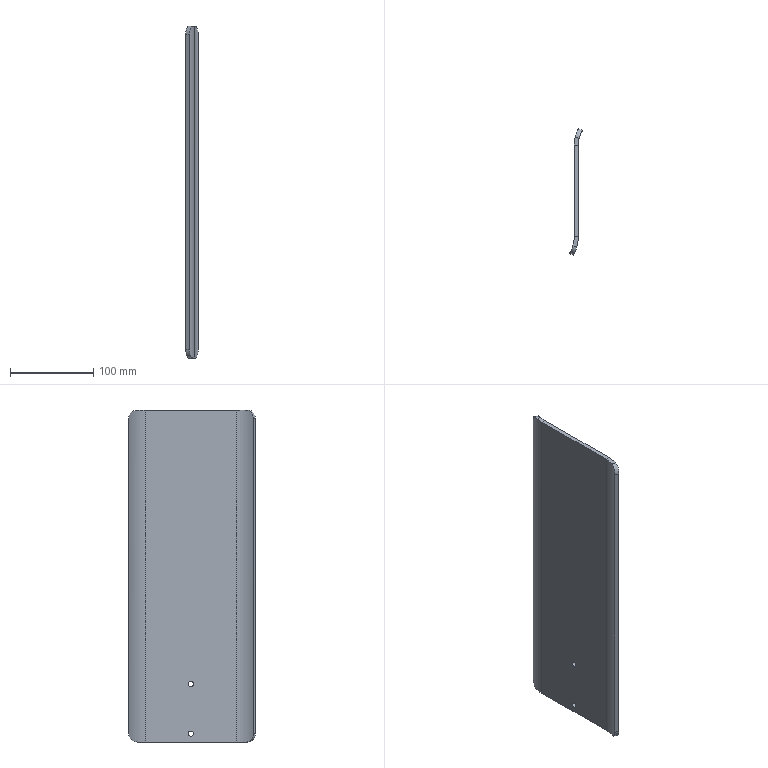Part | STEP file | Water guard plate SGN-7-02 | 1 solid | 22 faces | box 15.048 x 152.5 x 400 mm | volume 302987 mm3 | plane 10 | cylinder 8 | spline 4 | commonest cylinder face diameters 6.5 x4 80 x2 70 x1 90 x1